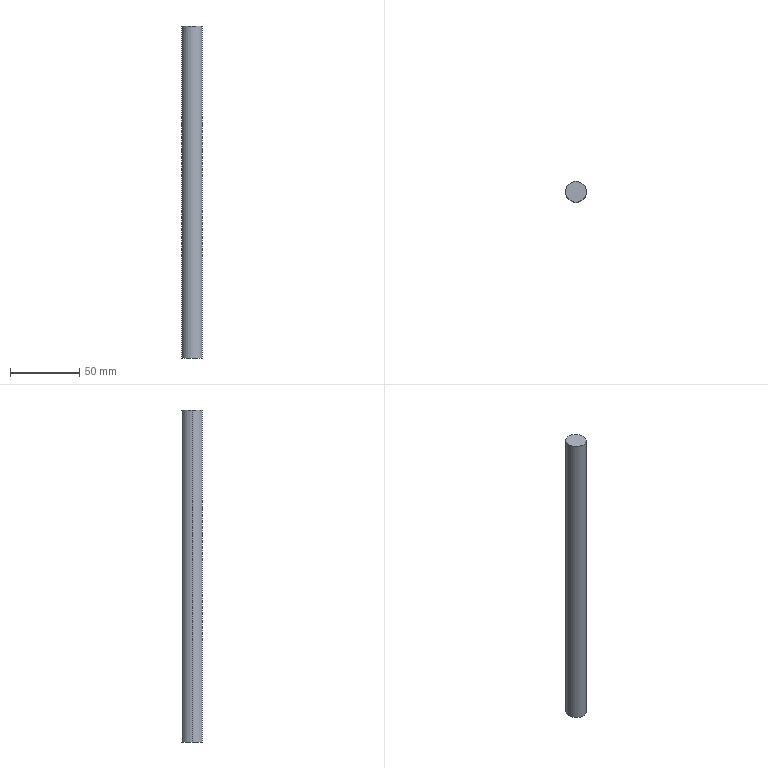Part | SolidWorks | features Extrusion 1 | 1 solid | 4 faces | box 15 x 15 x 240 mm | volume 42412 mm3 | cylinder 2 | plane 2 | commonest cylinder face diameters 15 x2
STEP:
#1=CARTESIAN_POINT('',(7.5,0.,240.));
#2=VERTEX_POINT('',#1);
#3=CARTESIAN_POINT('',(-7.5,0.,240.));
#4=VERTEX_POINT('',#3);
#5=CARTESIAN_POINT('',(0.,0.,240.));
#6=DIRECTION('',(0.,0.,1.));
#7=DIRECTION('',(1.,0.,0.));
#8=AXIS2_PLACEMENT_3D('',#5,#6,#7);
#9=CIRCLE('',#8,7.5);
#10=EDGE_CURVE('',#2,#4,#9,.T.);
#11=ORIENTED_EDGE('',*,*,#10,.F.);
#12=CARTESIAN_POINT('',(7.5,0.,0.));
#13=VERTEX_POINT('',#12);
#14=CARTESIAN_POINT('',(7.5,0.,240.));
#15=DIRECTION('',(0.,0.,-1.));
#16=VECTOR('',#15,1000.);
#17=LINE('',#14,#16);
#18=EDGE_CURVE('',#2,#13,#17,.T.);
#19=ORIENTED_EDGE('',*,*,#18,.T.);
#20=CARTESIAN_POINT('',(-7.5,0.,0.));
#21=VERTEX_POINT('',#20);
#22=CARTESIAN_POINT('',(0.,0.,0.));
#23=DIRECTION('',(0.,0.,1.));
#24=DIRECTION('',(1.,0.,0.));
#25=AXIS2_PLACEMENT_3D('',#22,#23,#24);
#26=CIRCLE('',#25,7.5);
#27=EDGE_CURVE('',#13,#21,#26,.T.);
#28=ORIENTED_EDGE('',*,*,#27,.T.);
#29=CARTESIAN_POINT('',(-7.5,0.,240.));
#30=DIRECTION('',(0.,0.,-1.));
#31=VECTOR('',#30,1000.);
#32=LINE('',#29,#31);
#33=EDGE_CURVE('',#4,#21,#32,.T.);
#34=ORIENTED_EDGE('',*,*,#33,.F.);
#35=EDGE_LOOP('',(#11,#19,#28,#34));
#36=FACE_OUTER_BOUND('',#35,.T.);
#37=CARTESIAN_POINT('',(0.,0.,240.));
#38=DIRECTION('',(0.,0.,-1.));
#39=DIRECTION('',(-1.,0.,0.));
#40=AXIS2_PLACEMENT_3D('',#37,#38,#39);
#41=CYLINDRICAL_SURFACE('',#40,7.5);
#42=ADVANCED_FACE('',(#36),#41,.T.);
#43=ORIENTED_EDGE('',*,*,#18,.F.);
#44=CARTESIAN_POINT('',(0.,0.,240.));
#45=DIRECTION('',(0.,0.,1.));
#46=DIRECTION('',(1.,0.,0.));
#47=AXIS2_PLACEMENT_3D('',#44,#45,#46);
#48=CIRCLE('',#47,7.5);
#49=EDGE_CURVE('',#4,#2,#48,.T.);
#50=ORIENTED_EDGE('',*,*,#49,.F.);
#51=ORIENTED_EDGE('',*,*,#33,.T.);
#52=CARTESIAN_POINT('',(0.,0.,0.));
#53=DIRECTION('',(0.,0.,1.));
#54=DIRECTION('',(1.,0.,0.));
#55=AXIS2_PLACEMENT_3D('',#52,#53,#54);
#56=CIRCLE('',#55,7.5);
#57=EDGE_CURVE('',#21,#13,#56,.T.);
#58=ORIENTED_EDGE('',*,*,#57,.T.);
#59=EDGE_LOOP('',(#43,#50,#51,#58));
#60=FACE_OUTER_BOUND('',#59,.T.);
#61=CARTESIAN_POINT('',(0.,0.,240.));
#62=DIRECTION('',(0.,0.,-1.));
#63=DIRECTION('',(-1.,0.,0.));
#64=AXIS2_PLACEMENT_3D('',#61,#62,#63);
#65=CYLINDRICAL_SURFACE('',#64,7.5);
#66=ADVANCED_FACE('',(#60),#65,.T.);
#67=ORIENTED_EDGE('',*,*,#49,.T.);
#68=ORIENTED_EDGE('',*,*,#10,.T.);
#69=EDGE_LOOP('',(#67,#68));
#70=FACE_OUTER_BOUND('',#69,.T.);
#71=CARTESIAN_POINT('',(0.,0.,240.));
#72=DIRECTION('',(0.,0.,1.));
#73=DIRECTION('',(1.,0.,0.));
#74=AXIS2_PLACEMENT_3D('',#71,#72,#73);
#75=PLANE('',#74);
#76=ADVANCED_FACE('',(#70),#75,.T.);
#77=ORIENTED_EDGE('',*,*,#57,.F.);
#78=ORIENTED_EDGE('',*,*,#27,.F.);
#79=EDGE_LOOP('',(#77,#78));
#80=FACE_OUTER_BOUND('',#79,.T.);
#81=CARTESIAN_POINT('',(0.,0.,0.));
#82=DIRECTION('',(0.,0.,1.));
#83=DIRECTION('',(1.,0.,0.));
#84=AXIS2_PLACEMENT_3D('',#81,#82,#83);
#85=PLANE('',#84);
#86=ADVANCED_FACE('',(#80),#85,.F.);
#87=CLOSED_SHELL('',(#42,#66,#76,#86));
#88=MANIFOLD_SOLID_BREP('',#87);
#89=CARTESIAN_POINT('',(0.,0.,0.));
#90=DIRECTION('',(0.,0.,1.));
#91=DIRECTION('',(1.,0.,0.));
#92=AXIS2_PLACEMENT_3D('',#89,#90,#91);
#93=(LENGTH_UNIT()NAMED_UNIT(*)SI_UNIT(.MILLI.,.METRE.));
#94=UNCERTAINTY_MEASURE_WITH_UNIT(LENGTH_MEASURE(0.00001),#93,'','');
#95=(NAMED_UNIT(*)PLANE_ANGLE_UNIT()SI_UNIT($,.RADIAN.));
#96=(NAMED_UNIT(*)SI_UNIT($,.STERADIAN.)SOLID_ANGLE_UNIT());
#97=(GEOMETRIC_REPRESENTATION_CONTEXT(3)GLOBAL_UNCERTAINTY_ASSIGNED_CONTEXT((#94))GLOBAL_UNIT_ASSIGNED_CONTEXT((#93,#95,#96))REPRESENTATION_CONTEXT('',''));
#98=ADVANCED_BREP_SHAPE_REPRESENTATION('',(#88,#92),#97);